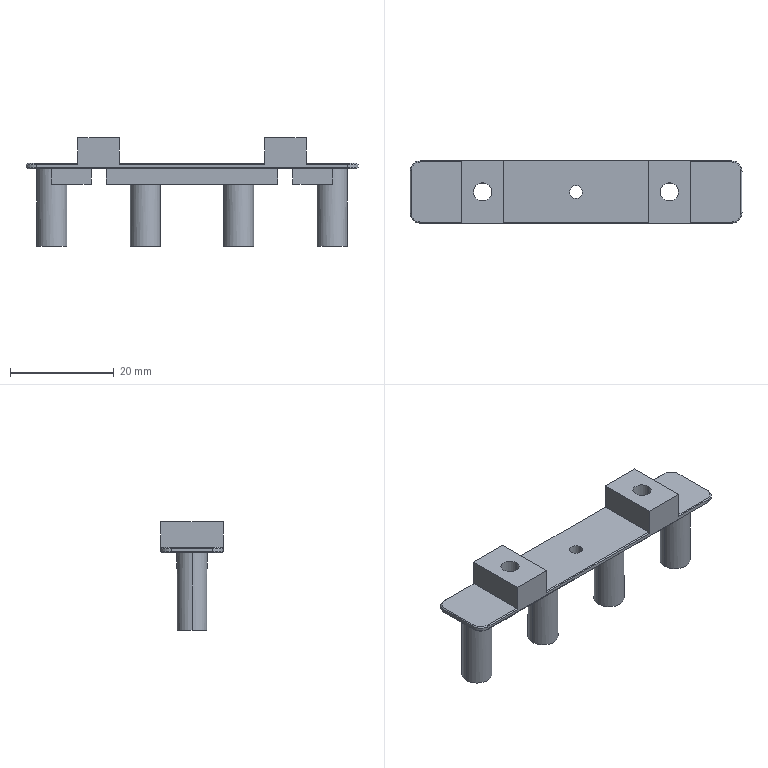NC program | NX | posted with a generic post | part box 64 x 12 x 21 mm
Lines 1 to 927 of 2253:
N10 G17 G21 G94 G90
(FLOOR_WALL_1_COPY_1 , TOOL : D10)
N12 T15 M6
N14 G54
N16 G17 G0 G90 X-0.866 Y8.55 S9500 M3
N18 G43 Z30. H15
N20 Z0.507
N22 G94 G1 Z-0.993 F2500.
N24 G3 X0. Y8.05 R1.
N26 G1 X16.533
N28 G2 X18. Y7.837 R5.15
N30 X19.467 Y8.05 R5.15
N32 G1 X27.
N34 G2 X35.05 Y0. R8.05
N36 X27. Y-8.05 R8.05
N38 G1 X19.467
N40 G2 X18. Y-7.837 R5.15
N42 X16.533 Y-8.05 R5.15
N44 G1 X-16.533
N46 G2 X-18. Y-7.837 R5.15
N48 X-19.467 Y-8.05 R5.15
N50 G1 X-27.
N52 G2 X-35.05 Y0. R8.05
N54 X-27. Y8.05 R8.05
N56 G1 X-19.467
N58 G2 X-18. Y7.837 R5.15
N60 X-16.533 Y8.05 R5.15
N62 G1 X0.
N64 G3 X0.866 Y8.55 R1.
N66 G1 Z0.507
N68 G0 X-0.866 Z-0.487
N70 G1 Z-1.987
N72 G3 X0. Y8.05 R1.
N74 G1 X16.533
N76 G2 X18. Y7.837 R5.15
N78 X19.467 Y8.05 R5.15
N80 G1 X27.
N82 G2 X35.05 Y0. R8.05
N84 X27. Y-8.05 R8.05
N86 G1 X19.467
N88 G2 X18. Y-7.837 R5.15
N90 X16.533 Y-8.05 R5.15
N92 G1 X-16.533
N94 G2 X-18. Y-7.837 R5.15
N96 X-19.467 Y-8.05 R5.15
N98 G1 X-27.
N100 G2 X-35.05 Y0. R8.05
N102 X-27. Y8.05 R8.05
N104 G1 X-19.467
N106 G2 X-18. Y7.837 R5.15
N108 X-16.533 Y8.05 R5.15
N110 G1 X0.
N112 G3 X0.866 Y8.55 R1.
N114 G1 Z-0.487
N116 G0 X-0.866 Z-1.48
N118 G1 Z-2.98
N120 G3 X0. Y8.05 R1.
N122 G1 X16.533
N124 G2 X18. Y7.837 R5.15
N126 X19.467 Y8.05 R5.15
N128 G1 X27.
N130 G2 X35.05 Y0. R8.05
N132 X27. Y-8.05 R8.05
N134 G1 X19.467
N136 G2 X18. Y-7.837 R5.15
N138 X16.533 Y-8.05 R5.15
N140 G1 X-16.533
N142 G2 X-18. Y-7.837 R5.15
N144 X-19.467 Y-8.05 R5.15
N146 G1 X-27.
N148 G2 X-35.05 Y0. R8.05
N150 X-27. Y8.05 R8.05
N152 G1 X-19.467
N154 G2 X-18. Y7.837 R5.15
N156 X-16.533 Y8.05 R5.15
N158 G1 X0.
N160 G3 X0.866 Y8.55 R1.
N162 G1 Z-1.48
N164 G0 X-0.866 Z-2.473
N166 G1 Z-3.973
N168 G3 X0. Y8.05 R1.
N170 G1 X16.533
N172 G2 X18. Y7.837 R5.15
N174 X19.467 Y8.05 R5.15
N176 G1 X27.
N178 G2 X35.05 Y0. R8.05
N180 X27. Y-8.05 R8.05
N182 G1 X19.467
N184 G2 X18. Y-7.837 R5.15
N186 X16.533 Y-8.05 R5.15
N188 G1 X-16.533
N190 G2 X-18. Y-7.837 R5.15
N192 X-19.467 Y-8.05 R5.15
N194 G1 X-27.
N196 G2 X-35.05 Y0. R8.05
N198 X-27. Y8.05 R8.05
N200 G1 X-19.467
N202 G2 X-18. Y7.837 R5.15
N204 X-16.533 Y8.05 R5.15
N206 G1 X0.
N208 G3 X0.866 Y8.55 R1.
N210 G1 Z-2.473
N212 G0 X-0.866 Z-3.467
N214 G1 Z-4.967
N216 G3 X0. Y8.05 R1.
N218 G1 X16.533
N220 G2 X18. Y7.837 R5.15
N222 X19.467 Y8.05 R5.15
N224 G1 X27.
N226 G2 X35.05 Y0. R8.05
N228 X27. Y-8.05 R8.05
N230 G1 X19.467
N232 G2 X18. Y-7.837 R5.15
N234 X16.533 Y-8.05 R5.15
N236 G1 X-16.533
N238 G2 X-18. Y-7.837 R5.15
N240 X-19.467 Y-8.05 R5.15
N242 G1 X-27.
N244 G2 X-35.05 Y0. R8.05
N246 X-27. Y8.05 R8.05
N248 G1 X-19.467
N250 G2 X-18. Y7.837 R5.15
N252 X-16.533 Y8.05 R5.15
N254 G1 X0.
N256 G3 X0.866 Y8.55 R1.
N258 G1 Z-3.467
N260 G0 X-0.866 Z-4.46
N262 G1 Z-5.96
N264 G3 X0. Y8.05 R1.
N266 G1 X16.533
N268 G2 X18. Y7.837 R5.15
N270 X19.467 Y8.05 R5.15
N272 G1 X27.
N274 G2 X35.05 Y0. R8.05
N276 X27. Y-8.05 R8.05
N278 G1 X19.467
N280 G2 X18. Y-7.837 R5.15
N282 X16.533 Y-8.05 R5.15
N284 G1 X-16.533
N286 G2 X-18. Y-7.837 R5.15
N288 X-19.467 Y-8.05 R5.15
N290 G1 X-27.
N292 G2 X-35.05 Y0. R8.05
N294 X-27. Y8.05 R8.05
N296 G1 X-19.467
N298 G2 X-18. Y7.837 R5.15
N300 X-16.533 Y8.05 R5.15
N302 G1 X0.
N304 G3 X0.866 Y8.55 R1.
N306 G1 Z-4.46
N308 G0 X-0.866 Z-5.453
N310 G1 Z-6.953
N312 G3 X0. Y8.05 R1.
N314 G1 X16.533
N316 G2 X18. Y7.837 R5.15
N318 X19.467 Y8.05 R5.15
N320 G1 X27.
N322 G2 X35.05 Y0. R8.05
N324 X27. Y-8.05 R8.05
N326 G1 X19.467
N328 G2 X18. Y-7.837 R5.15
N330 X16.533 Y-8.05 R5.15
N332 G1 X-16.533
N334 G2 X-18. Y-7.837 R5.15
N336 X-19.467 Y-8.05 R5.15
N338 G1 X-27.
N340 G2 X-35.05 Y0. R8.05
N342 X-27. Y8.05 R8.05
N344 G1 X-19.467
N346 G2 X-18. Y7.837 R5.15
N348 X-16.533 Y8.05 R5.15
N350 G1 X0.
N352 G3 X0.866 Y8.55 R1.
N354 G1 Z-5.453
N356 G0 X-0.866 Z-6.447
N358 G1 Z-7.947
N360 G3 X0. Y8.05 R1.
N362 G1 X16.533
N364 G2 X18. Y7.837 R5.15
N366 X19.467 Y8.05 R5.15
N368 G1 X27.
N370 G2 X35.05 Y0. R8.05
N372 X27. Y-8.05 R8.05
N374 G1 X19.467
N376 G2 X18. Y-7.837 R5.15
N378 X16.533 Y-8.05 R5.15
N380 G1 X-16.533
N382 G2 X-18. Y-7.837 R5.15
N384 X-19.467 Y-8.05 R5.15
N386 G1 X-27.
N388 G2 X-35.05 Y0. R8.05
N390 X-27. Y8.05 R8.05
N392 G1 X-19.467
N394 G2 X-18. Y7.837 R5.15
N396 X-16.533 Y8.05 R5.15
N398 G1 X0.
N400 G3 X0.866 Y8.55 R1.
N402 G1 Z-6.447
N404 G0 X-0.866 Z-7.44
N406 G1 Z-8.94
N408 G3 X0. Y8.05 R1.
N410 G1 X16.533
N412 G2 X18. Y7.837 R5.15
N414 X19.467 Y8.05 R5.15
N416 G1 X27.
N418 G2 X35.05 Y0. R8.05
N420 X27. Y-8.05 R8.05
N422 G1 X19.467
N424 G2 X18. Y-7.837 R5.15
N426 X16.533 Y-8.05 R5.15
N428 G1 X-16.533
N430 G2 X-18. Y-7.837 R5.15
N432 X-19.467 Y-8.05 R5.15
N434 G1 X-27.
N436 G2 X-35.05 Y0. R8.05
N438 X-27. Y8.05 R8.05
N440 G1 X-19.467
N442 G2 X-18. Y7.837 R5.15
N444 X-16.533 Y8.05 R5.15
N446 G1 X0.
N448 G3 X0.866 Y8.55 R1.
N450 G1 Z-7.44
N452 G0 X-0.866 Z-8.433
N454 G1 Z-9.933
N456 G3 X0. Y8.05 R1.
N458 G1 X16.533
N460 G2 X18. Y7.837 R5.15
N462 X19.467 Y8.05 R5.15
N464 G1 X27.
N466 G2 X35.05 Y0. R8.05
N468 X27. Y-8.05 R8.05
N470 G1 X19.467
N472 G2 X18. Y-7.837 R5.15
N474 X16.533 Y-8.05 R5.15
N476 G1 X-16.533
N478 G2 X-18. Y-7.837 R5.15
N480 X-19.467 Y-8.05 R5.15
N482 G1 X-27.
N484 G2 X-35.05 Y0. R8.05
N486 X-27. Y8.05 R8.05
N488 G1 X-19.467
N490 G2 X-18. Y7.837 R5.15
N492 X-16.533 Y8.05 R5.15
N494 G1 X0.
N496 G3 X0.866 Y8.55 R1.
N498 G1 Z-8.433
N500 G0 X-0.866 Z-9.427
N502 G1 Z-10.927
N504 G3 X0. Y8.05 R1.
N506 G1 X16.533
N508 G2 X18. Y7.837 R5.15
N510 X19.467 Y8.05 R5.15
N512 G1 X27.
N514 G2 X35.05 Y0. R8.05
N516 X27. Y-8.05 R8.05
N518 G1 X19.467
N520 G2 X18. Y-7.837 R5.15
N522 X16.533 Y-8.05 R5.15
N524 G1 X-16.533
N526 G2 X-18. Y-7.837 R5.15
N528 X-19.467 Y-8.05 R5.15
N530 G1 X-27.
N532 G2 X-35.05 Y0. R8.05
N534 X-27. Y8.05 R8.05
N536 G1 X-19.467
N538 G2 X-18. Y7.837 R5.15
N540 X-16.533 Y8.05 R5.15
N542 G1 X0.
N544 G3 X0.866 Y8.55 R1.
N546 G1 Z-9.427
N548 G0 X-0.866 Z-10.42
N550 G1 Z-11.92
N552 G3 X0. Y8.05 R1.
N554 G1 X16.533
N556 G2 X18. Y7.837 R5.15
N558 X19.467 Y8.05 R5.15
N560 G1 X27.
N562 G2 X35.05 Y0. R8.05
N564 X27. Y-8.05 R8.05
N566 G1 X19.467
N568 G2 X18. Y-7.837 R5.15
N570 X16.533 Y-8.05 R5.15
N572 G1 X-16.533
N574 G2 X-18. Y-7.837 R5.15
N576 X-19.467 Y-8.05 R5.15
N578 G1 X-27.
N580 G2 X-35.05 Y0. R8.05
N582 X-27. Y8.05 R8.05
N584 G1 X-19.467
N586 G2 X-18. Y7.837 R5.15
N588 X-16.533 Y8.05 R5.15
N590 G1 X0.
N592 G3 X0.866 Y8.55 R1.
N594 G1 Z-10.42
N596 G0 X-1.443 Y9.55 Z-11.413
N598 G1 Z-12.913
N600 X-0.866 Y8.55
N602 G3 X0. Y8.05 R1.
N604 G1 X16.533
N606 G2 X18. Y7.837 R5.15
N608 X19.467 Y8.05 R5.15
N610 G1 X27.
N612 G2 X35.05 Y0. R8.05
N614 X27. Y-8.05 R8.05
N616 G1 X19.467
N618 G2 X18. Y-7.837 R5.15
N620 X16.533 Y-8.05 R5.15
N622 G1 X-16.533
N624 G2 X-18. Y-7.837 R5.15
N626 X-19.467 Y-8.05 R5.15
N628 G1 X-27.
N630 G2 X-35.05 Y0. R8.05
N632 X-27. Y8.05 R8.05
N634 G1 X-19.467
N636 G2 X-18. Y7.837 R5.15
N638 X-16.533 Y8.05 R5.15
N640 G1 X0.
N642 G3 X0.866 Y8.55 R1.
N644 G1 X1.443 Y9.55
N646 Z-11.413
N648 G0 X-1.443 Z-12.407
N650 G1 Z-13.907
N652 X-0.866 Y8.55
N654 G3 X0. Y8.05 R1.
N656 G1 X16.533
N658 G2 X18. Y7.837 R5.15
N660 X19.467 Y8.05 R5.15
N662 G1 X27.
N664 G2 X35.05 Y0. R8.05
N666 X27. Y-8.05 R8.05
N668 G1 X19.467
N670 G2 X18. Y-7.837 R5.15
N672 X16.533 Y-8.05 R5.15
N674 G1 X-16.533
N676 G2 X-18. Y-7.837 R5.15
N678 X-19.467 Y-8.05 R5.15
N680 G1 X-27.
N682 G2 X-35.05 Y0. R8.05
N684 X-27. Y8.05 R8.05
N686 G1 X-19.467
N688 G2 X-18. Y7.837 R5.15
N690 X-16.533 Y8.05 R5.15
N692 G1 X0.
N694 G3 X0.866 Y8.55 R1.
N696 G1 X1.443 Y9.55
N698 Z-12.407
N700 G0 X-1.443 Z-13.4
N702 G1 Z-14.9
N704 X-0.866 Y8.55
N706 G3 X0. Y8.05 R1.
N708 G1 X16.533
N710 G2 X18. Y7.837 R5.15
N712 X19.467 Y8.05 R5.15
N714 G1 X27.
N716 G2 X35.05 Y0. R8.05
N718 X27. Y-8.05 R8.05
N720 G1 X19.467
N722 G2 X18. Y-7.837 R5.15
N724 X16.533 Y-8.05 R5.15
N726 G1 X-16.533
N728 G2 X-18. Y-7.837 R5.15
N730 X-19.467 Y-8.05 R5.15
N732 G1 X-27.
N734 G2 X-35.05 Y0. R8.05
N736 X-27. Y8.05 R8.05
N738 G1 X-19.467
N740 G2 X-18. Y7.837 R5.15
N742 X-16.533 Y8.05 R5.15
N744 G1 X0.
N746 G3 X0.866 Y8.55 R1.
N748 G1 X1.443 Y9.55
N750 Z-13.4
N752 G0 Z30.
(FLOOR_WALL_1_COPY_1_COPY , TOOL : D10)
N754 X-16.557 Y-9.4
N756 Z3.507
N758 G1 Z2.007
N760 X-17.134 Y-8.4
N762 G3 X-18. Y-7.9 R1.
N764 G1 X-25.453
N766 G3 X-25.453 Y7.9 R8.05
N768 G1 X-10.547
N770 G3 X-10.547 Y-7.9 R8.05
N772 G1 X-18.
N774 G3 X-18.866 Y-8.4 R1.
N776 G1 X-19.443 Y-9.4
N778 Z3.507
N780 G0 X-16.557 Z2.513
N782 G1 Z1.013
N784 X-17.134 Y-8.4
N786 G3 X-18. Y-7.9 R1.
N788 G1 X-25.453
N790 G3 X-25.453 Y7.9 R8.05
N792 G1 X-10.547
N794 G3 X-10.547 Y-7.9 R8.05
N796 G1 X-18.
N798 G3 X-18.866 Y-8.4 R1.
N800 G1 X-19.443 Y-9.4
N802 Z2.513
N804 G0 X-16.557 Z1.52
N806 G1 Z0.02
N808 X-17.134 Y-8.4
N810 G3 X-18. Y-7.9 R1.
N812 G1 X-25.453
N814 G3 X-25.453 Y7.9 R8.05
N816 G1 X-10.547
N818 G3 X-10.547 Y-7.9 R8.05
N820 G1 X-18.
N822 G3 X-18.866 Y-8.4 R1.
N824 G1 X-19.443 Y-9.4
N826 Z1.52
N828 G0 X-16.557 Z0.527
N830 G1 Z-0.973
N832 X-17.134 Y-8.4
N834 G3 X-18. Y-7.9 R1.
N836 G1 X-25.453
N838 G3 X-25.453 Y7.9 R8.05
N840 G1 X-10.547
N842 G3 X-10.547 Y-7.9 R8.05
N844 G1 X-18.
N846 G3 X-18.866 Y-8.4 R1.
N848 G1 X-19.443 Y-9.4
N850 Z0.527
N852 G0 X-16.557 Z-0.467
N854 G1 Z-1.967
N856 X-17.134 Y-8.4
N858 G3 X-18. Y-7.9 R1.
N860 G1 X-25.453
N862 G3 X-25.453 Y7.9 R8.05
N864 G1 X-10.547
N866 G3 X-10.547 Y-7.9 R8.05
N868 G1 X-18.
N870 G3 X-18.866 Y-8.4 R1.
N872 G1 X-19.443 Y-9.4
N874 Z-0.467
N876 G0 X-16.557 Z-1.46
N878 G1 Z-2.96
N880 X-17.134 Y-8.4
N882 G3 X-18. Y-7.9 R1.
N884 G1 X-25.453
N886 G3 X-25.453 Y7.9 R8.05
N888 G1 X-10.547
N890 G3 X-10.547 Y-7.9 R8.05
N892 G1 X-18.
N894 G3 X-18.866 Y-8.4 R1.
N896 G1 X-19.443 Y-9.4
N898 Z-1.46
N900 G0 X-16.557 Z-2.453
N902 G1 Z-3.953
N904 X-17.134 Y-8.4
N906 G3 X-18. Y-7.9 R1.
N908 G1 X-25.453
N910 G3 X-25.453 Y7.9 R8.05
N912 G1 X-10.547
N914 G3 X-10.547 Y-7.9 R8.05
N916 G1 X-18.
N918 G3 X-18.866 Y-8.4 R1.
N920 G1 X-19.443 Y-9.4
N922 Z-2.453
N924 G0 X-16.557 Z-3.447
N926 G1 Z-4.947
N928 X-17.134 Y-8.4
N930 G3 X-18. Y-7.9 R1.
N932 G1 X-25.453
N934 G3 X-25.453 Y7.9 R8.05
N936 G1 X-10.547
N938 G3 X-10.547 Y-7.9 R8.05
N940 G1 X-18.
N942 G3 X-18.866 Y-8.4 R1.
N944 G1 X-19.443 Y-9.4
N946 Z-3.447
N948 G0 X-16.557 Z-4.44
N950 G1 Z-5.94
N952 X-17.134 Y-8.4
N954 G3 X-18. Y-7.9 R1.
N956 G1 X-25.453
N958 G3 X-25.453 Y7.9 R8.05
N960 G1 X-10.547
N962 G3 X-10.547 Y-7.9 R8.05
N964 G1 X-18.
N966 G3 X-18.866 Y-8.4 R1.
N968 G1 X-19.443 Y-9.4
N970 Z-4.44
N972 G0 X-16.557 Z-5.433
N974 G1 Z-6.933
N976 X-17.134 Y-8.4
N978 G3 X-18. Y-7.9 R1.
N980 G1 X-25.453
N982 G3 X-25.453 Y7.9 R8.05
N984 G1 X-10.547
N986 G3 X-10.547 Y-7.9 R8.05
N988 G1 X-18.
N990 G3 X-18.866 Y-8.4 R1.
N992 G1 X-19.443 Y-9.4
N994 Z-5.433
N996 G0 X-16.557 Z-6.427
N998 G1 Z-7.927
N1000 X-17.134 Y-8.4
N1002 G3 X-18. Y-7.9 R1.
N1004 G1 X-25.453
N1006 G3 X-25.453 Y7.9 R8.05
N1008 G1 X-10.547
N1010 G3 X-10.547 Y-7.9 R8.05
N1012 G1 X-18.
N1014 G3 X-18.866 Y-8.4 R1.
N1016 G1 X-19.443 Y-9.4
N1018 Z-6.427
N1020 G0 X-16.557 Z-7.42
N1022 G1 Z-8.92
N1024 X-17.134 Y-8.4
N1026 G3 X-18. Y-7.9 R1.
N1028 G1 X-25.453
N1030 G3 X-25.453 Y7.9 R8.05
N1032 G1 X-10.547
N1034 G3 X-10.547 Y-7.9 R8.05
N1036 G1 X-18.
N1038 G3 X-18.866 Y-8.4 R1.
N1040 G1 X-19.443 Y-9.4
N1042 Z-7.42
N1044 G0 X-16.557 Z-8.413
N1046 G1 Z-9.913
N1048 X-17.134 Y-8.4
N1050 G3 X-18. Y-7.9 R1.
N1052 G1 X-25.453
N1054 G3 X-25.453 Y7.9 R8.05
N1056 G1 X-10.547
N1058 G3 X-10.547 Y-7.9 R8.05
N1060 G1 X-18.
N1062 G3 X-18.866 Y-8.4 R1.
N1064 G1 X-19.443 Y-9.4
N1066 Z-8.413
N1068 G0 X-16.557 Z-9.407
N1070 G1 Z-10.907
N1072 X-17.134 Y-8.4
N1074 G3 X-18. Y-7.9 R1.
N1076 G1 X-25.453
N1078 G3 X-25.453 Y7.9 R8.05
N1080 G1 X-10.547
N1082 G3 X-10.547 Y-7.9 R8.05
N1084 G1 X-18.
N1086 G3 X-18.866 Y-8.4 R1.
N1088 G1 X-19.443 Y-9.4
N1090 Z-9.407
N1092 G0 X-16.557 Z-10.4
N1094 G1 Z-11.9
N1096 X-17.134 Y-8.4
N1098 G3 X-18. Y-7.9 R1.
N1100 G1 X-25.453
N1102 G3 X-25.453 Y7.9 R8.05
N1104 G1 X-10.547
N1106 G3 X-10.547 Y-7.9 R8.05
N1108 G1 X-18.
N1110 G3 X-18.866 Y-8.4 R1.
N1112 G1 X-19.443 Y-9.4
N1114 Z-10.4
N1116 G0 Z30.
N1118 X1.443
N1120 Z3.507
N1122 G1 Z2.007
N1124 X0.866 Y-8.4
N1126 G3 X0. Y-7.9 R1.
N1128 G1 X-7.453
N1130 G3 X-7.453 Y7.9 R8.05
N1132 G1 X7.453
N1134 G3 X7.453 Y-7.9 R8.05
N1136 G1 X0.
N1138 G3 X-0.866 Y-8.4 R1.
N1140 G1 X-1.443 Y-9.4
N1142 Z3.507
N1144 G0 X1.443 Z2.513
N1146 G1 Z1.013
N1148 X0.866 Y-8.4
N1150 G3 X0. Y-7.9 R1.
N1152 G1 X-7.453
N1154 G3 X-7.453 Y7.9 R8.05
N1156 G1 X7.453
N1158 G3 X7.453 Y-7.9 R8.05
N1160 G1 X0.
N1162 G3 X-0.866 Y-8.4 R1.
N1164 G1 X-1.443 Y-9.4
N1166 Z2.513
N1168 G0 X1.443 Z1.52
N1170 G1 Z0.02
N1172 X0.866 Y-8.4
N1174 G3 X0. Y-7.9 R1.
N1176 G1 X-7.453
N1178 G3 X-7.453 Y7.9 R8.05
N1180 G1 X7.453
N1182 G3 X7.453 Y-7.9 R8.05
N1184 G1 X0.
N1186 G3 X-0.866 Y-8.4 R1.
N1188 G1 X-1.443 Y-9.4
N1190 Z1.52
N1192 G0 X1.443 Z0.527
N1194 G1 Z-0.973
N1196 X0.866 Y-8.4
N1198 G3 X0. Y-7.9 R1.
N1200 G1 X-7.453
N1202 G3 X-7.453 Y7.9 R8.05
N1204 G1 X7.453
N1206 G3 X7.453 Y-7.9 R8.05
N1208 G1 X0.
N1210 G3 X-0.866 Y-8.4 R1.
N1212 G1 X-1.443 Y-9.4
N1214 Z0.527
N1216 G0 X1.443 Z-0.467
N1218 G1 Z-1.967
N1220 X0.866 Y-8.4
N1222 G3 X0. Y-7.9 R1.
N1224 G1 X-7.453
N1226 G3 X-7.453 Y7.9 R8.05
N1228 G1 X7.453
N1230 G3 X7.453 Y-7.9 R8.05
N1232 G1 X0.
N1234 G3 X-0.866 Y-8.4 R1.
N1236 G1 X-1.443 Y-9.4
N1238 Z-0.467
N1240 G0 X1.443 Z-1.46
N1242 G1 Z-2.96
N1244 X0.866 Y-8.4
N1246 G3 X0. Y-7.9 R1.
N1248 G1 X-7.453
N1250 G3 X-7.453 Y7.9 R8.05
N1252 G1 X7.453
N1254 G3 X7.453 Y-7.9 R8.05
N1256 G1 X0.
N1258 G3 X-0.866 Y-8.4 R1.
N1260 G1 X-1.443 Y-9.4
N1262 Z-1.46
N1264 G0 X1.443 Z-2.453
N1266 G1 Z-3.953
N1268 X0.866 Y-8.4
N1270 G3 X0. Y-7.9 R1.
N1272 G1 X-7.453
N1274 G3 X-7.453 Y7.9 R8.05
N1276 G1 X7.453
N1278 G3 X7.453 Y-7.9 R8.05
N1280 G1 X0.
N1282 G3 X-0.866 Y-8.4 R1.
N1284 G1 X-1.443 Y-9.4
N1286 Z-2.453
N1288 G0 X1.443 Z-3.447
N1290 G1 Z-4.947
N1292 X0.866 Y-8.4
N1294 G3 X0. Y-7.9 R1.
N1296 G1 X-7.453
N1298 G3 X-7.453 Y7.9 R8.05
N1300 G1 X7.453
N1302 G3 X7.453 Y-7.9 R8.05
N1304 G1 X0.
N1306 G3 X-0.866 Y-8.4 R1.
N1308 G1 X-1.443 Y-9.4
N1310 Z-3.447
N1312 G0 X1.443 Z-4.44
N1314 G1 Z-5.94
N1316 X0.866 Y-8.4
N1318 G3 X0. Y-7.9 R1.
N1320 G1 X-7.453
N1322 G3 X-7.453 Y7.9 R8.05
N1324 G1 X7.453
N1326 G3 X7.453 Y-7.9 R8.05
N1328 G1 X0.
N1330 G3 X-0.866 Y-8.4 R1.
N1332 G1 X-1.443 Y-9.4
N1334 Z-4.44
N1336 G0 X1.443 Z-5.433
N1338 G1 Z-6.933
N1340 X0.866 Y-8.4
N1342 G3 X0. Y-7.9 R1.
N1344 G1 X-7.453
N1346 G3 X-7.453 Y7.9 R8.05
N1348 G1 X7.453
N1350 G3 X7.453 Y-7.9 R8.05
N1352 G1 X0.
N1354 G3 X-0.866 Y-8.4 R1.
N1356 G1 X-1.443 Y-9.4
N1358 Z-5.433
N1360 G0 X1.443 Z-6.427
N1362 G1 Z-7.927
N1364 X0.866 Y-8.4
N1366 G3 X0. Y-7.9 R1.
N1368 G1 X-7.453
N1370 G3 X-7.453 Y7.9 R8.05
N1372 G1 X7.453
N1374 G3 X7.453 Y-7.9 R8.05
N1376 G1 X0.
N1378 G3 X-0.866 Y-8.4 R1.
N1380 G1 X-1.443 Y-9.4
N1382 Z-6.427
N1384 G0 X1.443 Z-7.42
N1386 G1 Z-8.92
N1388 X0.866 Y-8.4
N1390 G3 X0. Y-7.9 R1.
N1392 G1 X-7.453
N1394 G3 X-7.453 Y7.9 R8.05
N1396 G1 X7.453
N1398 G3 X7.453 Y-7.9 R8.05
N1400 G1 X0.
N1402 G3 X-0.866 Y-8.4 R1.
N1404 G1 X-1.443 Y-9.4
N1406 Z-7.42
N1408 G0 X1.443 Z-8.413
N1410 G1 Z-9.913
N1412 X0.866 Y-8.4
N1414 G3 X0. Y-7.9 R1.
N1416 G1 X-7.453
N1418 G3 X-7.453 Y7.9 R8.05
N1420 G1 X7.453
N1422 G3 X7.453 Y-7.9 R8.05
N1424 G1 X0.
N1426 G3 X-0.866 Y-8.4 R1.
N1428 G1 X-1.443 Y-9.4
N1430 Z-8.413
N1432 G0 X1.443 Z-9.407
N1434 G1 Z-10.907
N1436 X0.866 Y-8.4
N1438 G3 X0. Y-7.9 R1.
N1440 G1 X-7.453
N1442 G3 X-7.453 Y7.9 R8.05
N1444 G1 X7.453
N1446 G3 X7.453 Y-7.9 R8.05
N1448 G1 X0.
N1450 G3 X-0.866 Y-8.4 R1.
N1452 G1 X-1.443 Y-9.4
N1454 Z-9.407
N1456 G0 X1.443 Z-10.4
N1458 G1 Z-11.9
N1460 X0.866 Y-8.4
N1462 G3 X0. Y-7.9 R1.
N1464 G1 X-7.453
N1466 G3 X-7.453 Y7.9 R8.05
N1468 G1 X7.453
N1470 G3 X7.453 Y-7.9 R8.05
N1472 G1 X0.
N1474 G3 X-0.866 Y-8.4 R1.
N1476 G1 X-1.443 Y-9.4
N1478 Z-10.4
N1480 G0 Z30.
N1482 X19.443
N1484 Z3.507
N1486 G1 Z2.007
N1488 X18.866 Y-8.4
N1490 G3 X18. Y-7.9 R1.
N1492 G1 X10.547
N1494 G3 X10.547 Y7.9 R8.05
N1496 G1 X25.453
N1498 G3 X25.453 Y-7.9 R8.05
N1500 G1 X18.
N1502 G3 X17.134 Y-8.4 R1.
N1504 G1 X16.557 Y-9.4
N1506 Z3.507
N1508 G0 X19.443 Z2.513
N1510 G1 Z1.013
N1512 X18.866 Y-8.4
N1514 G3 X18. Y-7.9 R1.
N1516 G1 X10.547
N1518 G3 X10.547 Y7.9 R8.05
N1520 G1 X25.453
N1522 G3 X25.453 Y-7.9 R8.05
N1524 G1 X18.
N1526 G3 X17.134 Y-8.4 R1.
N1528 G1 X16.557 Y-9.4
N1530 Z2.513
N1532 G0 X19.443 Z1.52
N1534 G1 Z0.02
N1536 X18.866 Y-8.4
N1538 G3 X18. Y-7.9 R1.
N1540 G1 X10.547
N1542 G3 X10.547 Y7.9 R8.05
N1544 G1 X25.453
N1546 G3 X25.453 Y-7.9 R8.05
N1548 G1 X18.
N1550 G3 X17.134 Y-8.4 R1.
N1552 G1 X16.557 Y-9.4
N1554 Z1.52
N1556 G0 X19.443 Z0.527
N1558 G1 Z-0.973
N1560 X18.866 Y-8.4
N1562 G3 X18. Y-7.9 R1.
N1564 G1 X10.547
N1566 G3 X10.547 Y7.9 R8.05
N1568 G1 X25.453
N1570 G3 X25.453 Y-7.9 R8.05
N1572 G1 X18.
N1574 G3 X17.134 Y-8.4 R1.
N1576 G1 X16.557 Y-9.4
N1578 Z0.527
N1580 G0 X19.443 Z-0.467
N1582 G1 Z-1.967
N1584 X18.866 Y-8.4
N1586 G3 X18. Y-7.9 R1.
N1588 G1 X10.547
N1590 G3 X10.547 Y7.9 R8.05
N1592 G1 X25.453
N1594 G3 X25.453 Y-7.9 R8.05
N1596 G1 X18.
N1598 G3 X17.134 Y-8.4 R1.
N1600 G1 X16.557 Y-9.4
N1602 Z-0.467
N1604 G0 X19.443 Z-1.46
N1606 G1 Z-2.96
N1608 X18.866 Y-8.4
N1610 G3 X18. Y-7.9 R1.
N1612 G1 X10.547
N1614 G3 X10.547 Y7.9 R8.05
N1616 G1 X25.453
N1618 G3 X25.453 Y-7.9 R8.05
N1620 G1 X18.
N1622 G3 X17.134 Y-8.4 R1.
N1624 G1 X16.557 Y-9.4
N1626 Z-1.46
N1628 G0 X19.443 Z-2.453
N1630 G1 Z-3.953
N1632 X18.866 Y-8.4
N1634 G3 X18. Y-7.9 R1.
N1636 G1 X10.547
N1638 G3 X10.547 Y7.9 R8.05
N1640 G1 X25.453
N1642 G3 X25.453 Y-7.9 R8.05
N1644 G1 X18.
N1646 G3 X17.134 Y-8.4 R1.
N1648 G1 X16.557 Y-9.4
N1650 Z-2.453
N1652 G0 X19.443 Z-3.447
N1654 G1 Z-4.947
N1656 X18.866 Y-8.4
N1658 G3 X18. Y-7.9 R1.
N1660 G1 X10.547
N1662 G3 X10.547 Y7.9 R8.05
N1664 G1 X25.453
N1666 G3 X25.453 Y-7.9 R8.05
N1668 G1 X18.
N1670 G3 X17.134 Y-8.4 R1.
N1672 G1 X16.557 Y-9.4
N1674 Z-3.447
N1676 G0 X19.443 Z-4.44
N1678 G1 Z-5.94
N1680 X18.866 Y-8.4
N1682 G3 X18. Y-7.9 R1.
N1684 G1 X10.547
N1686 G3 X10.547 Y7.9 R8.05
N1688 G1 X25.453
N1690 G3 X25.453 Y-7.9 R8.05
N1692 G1 X18.
N1694 G3 X17.134 Y-8.4 R1.
N1696 G1 X16.557 Y-9.4
N1698 Z-4.44
N1700 G0 X19.443 Z-5.433
N1702 G1 Z-6.933
N1704 X18.866 Y-8.4
N1706 G3 X18. Y-7.9 R1.
N1708 G1 X10.547
N1710 G3 X10.547 Y7.9 R8.05
N1712 G1 X25.453
N1714 G3 X25.453 Y-7.9 R8.05
N1716 G1 X18.
N1718 G3 X17.134 Y-8.4 R1.
N1720 G1 X16.557 Y-9.4
N1722 Z-5.433
N1724 G0 X19.443 Z-6.427
N1726 G1 Z-7.927
N1728 X18.866 Y-8.4
N1730 G3 X18. Y-7.9 R1.
N1732 G1 X10.547
N1734 G3 X10.547 Y7.9 R8.05
N1736 G1 X25.453
N1738 G3 X25.453 Y-7.9 R8.05
N1740 G1 X18.
N1742 G3 X17.134 Y-8.4 R1.
N1744 G1 X16.557 Y-9.4
N1746 Z-6.427
N1748 G0 X19.443 Z-7.42
N1750 G1 Z-8.92
N1752 X18.866 Y-8.4
N1754 G3 X18. Y-7.9 R1.
N1756 G1 X10.547
N1758 G3 X10.547 Y7.9 R8.05
N1760 G1 X25.453
N1762 G3 X25.453 Y-7.9 R8.05
N1764 G1 X18.
N1766 G3 X17.134 Y-8.4 R1.
N1768 G1 X16.557 Y-9.4
N1770 Z-7.42
N1772 G0 X19.443 Z-8.413
N1774 G1 Z-9.913
N1776 X18.866 Y-8.4
N1778 G3 X18. Y-7.9 R1.
N1780 G1 X10.547
N1782 G3 X10.547 Y7.9 R8.05
N1784 G1 X25.453
N1786 G3 X25.453 Y-7.9 R8.05
N1788 G1 X18.
N1790 G3 X17.134 Y-8.4 R1.
N1792 G1 X16.557 Y-9.4
N1794 Z-8.413
N1796 G0 X19.443 Z-9.407
N1798 G1 Z-10.907
N1800 X18.866 Y-8.4
N1802 G3 X18. Y-7.9 R1.
N1804 G1 X10.547
N1806 G3 X10.547 Y7.9 R8.05
N1808 G1 X25.453
N1810 G3 X25.453 Y-7.9 R8.05
N1812 G1 X18.
N1814 G3 X17.134 Y-8.4 R1.
N1816 G1 X16.557 Y-9.4
N1818 Z-9.407
N1820 G0 X19.443 Z-10.4
N1822 G1 Z-11.9
N1824 X18.866 Y-8.4
N1826 G3 X18. Y-7.9 R1.
N1828 G1 X10.547
N1830 G3 X10.547 Y7.9 R8.05
N1832 G1 X25.453
N1834 G3 X25.453 Y-7.9 R8.05
N1836 G1 X18.
N1838 G3 X17.134 Y-8.4 R1.
N1840 G1 X16.557 Y-9.4
N1842 Z-10.4
N1844 G0 Z30.
N1846 M5